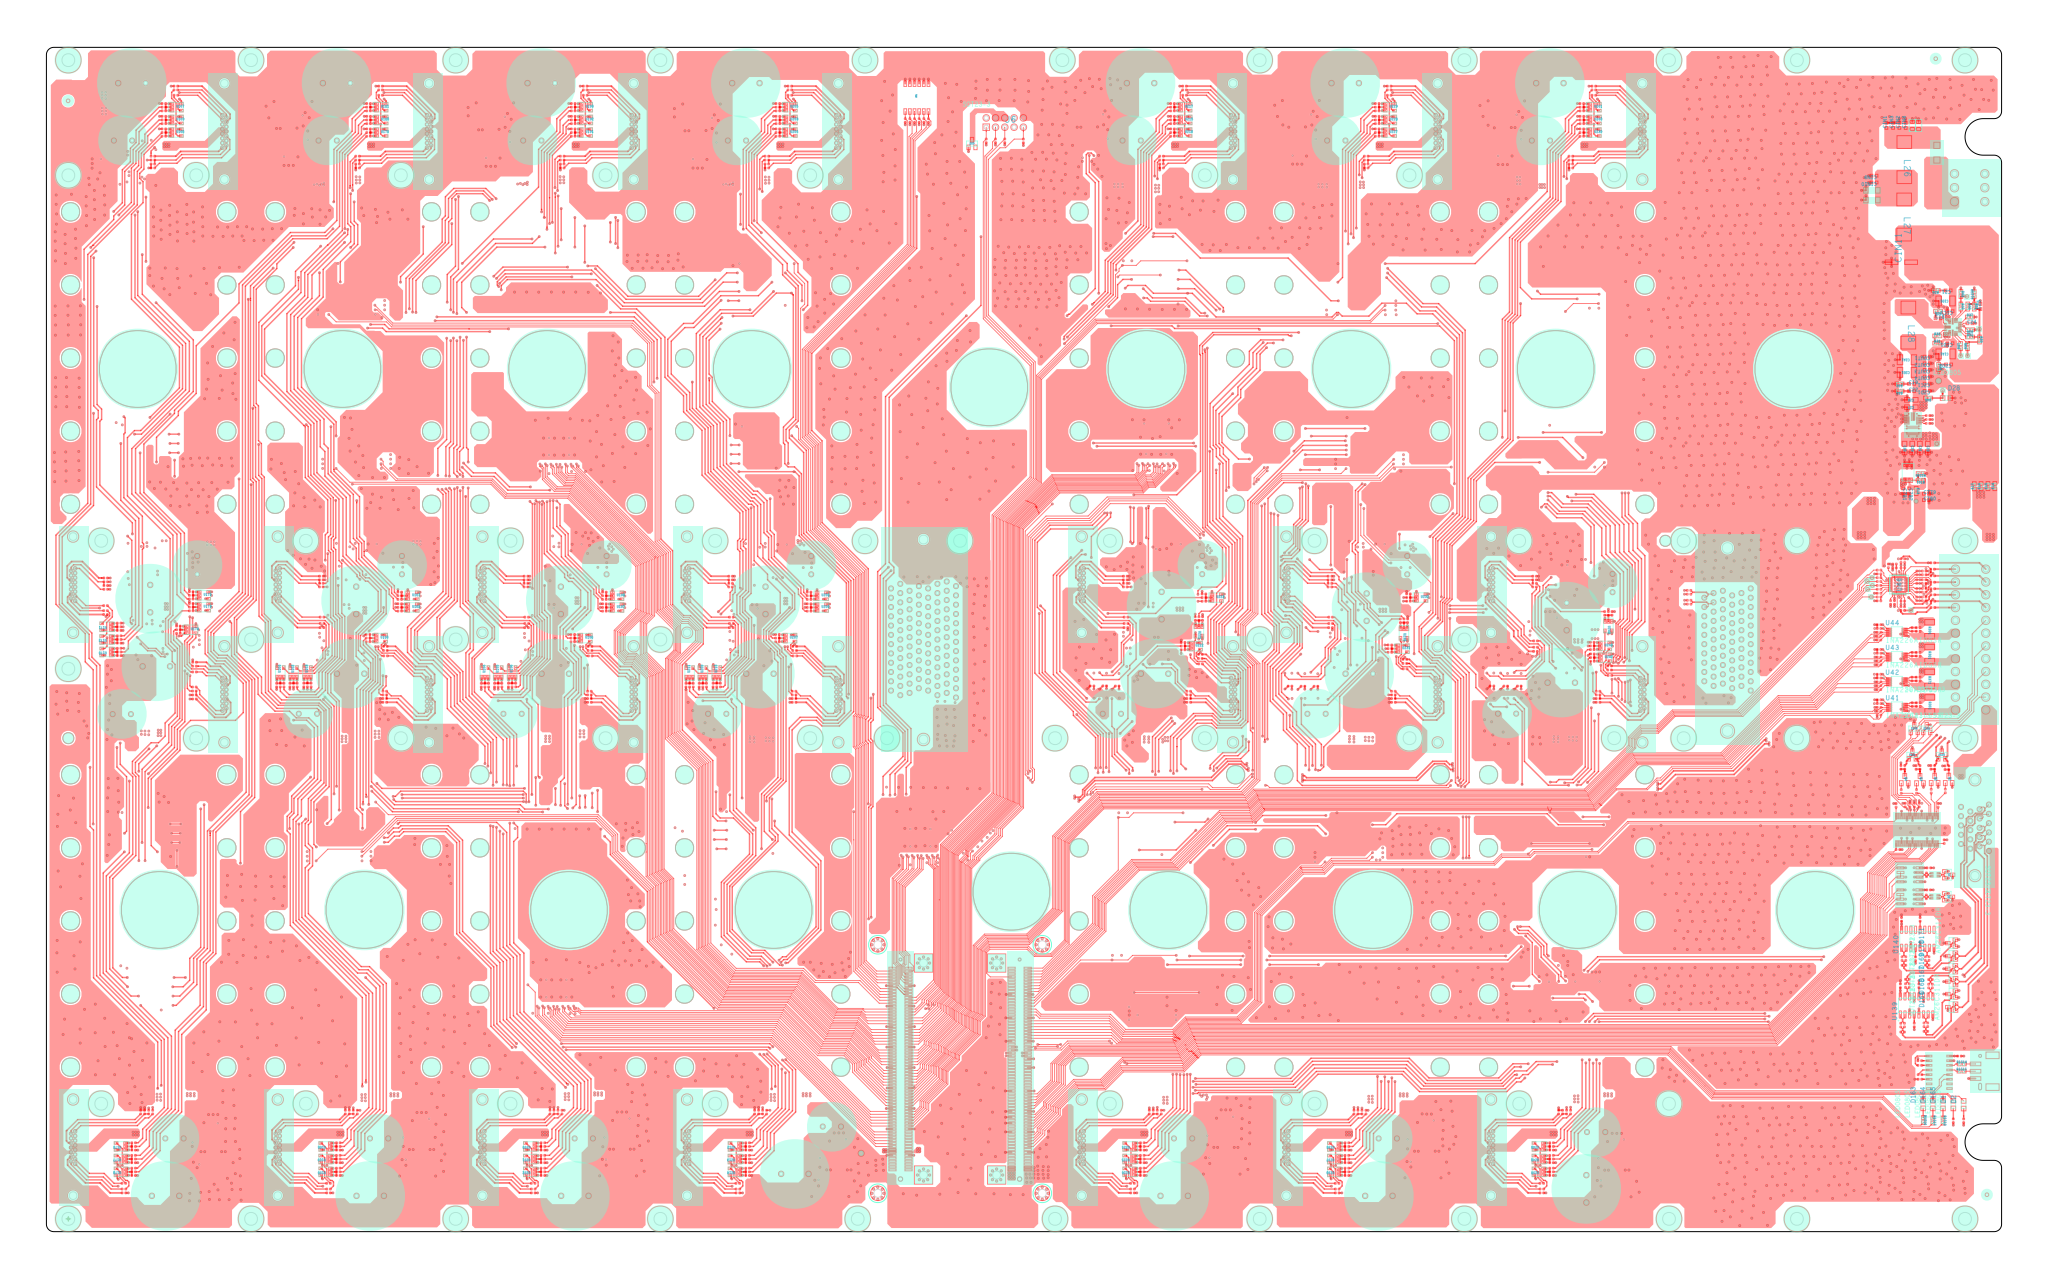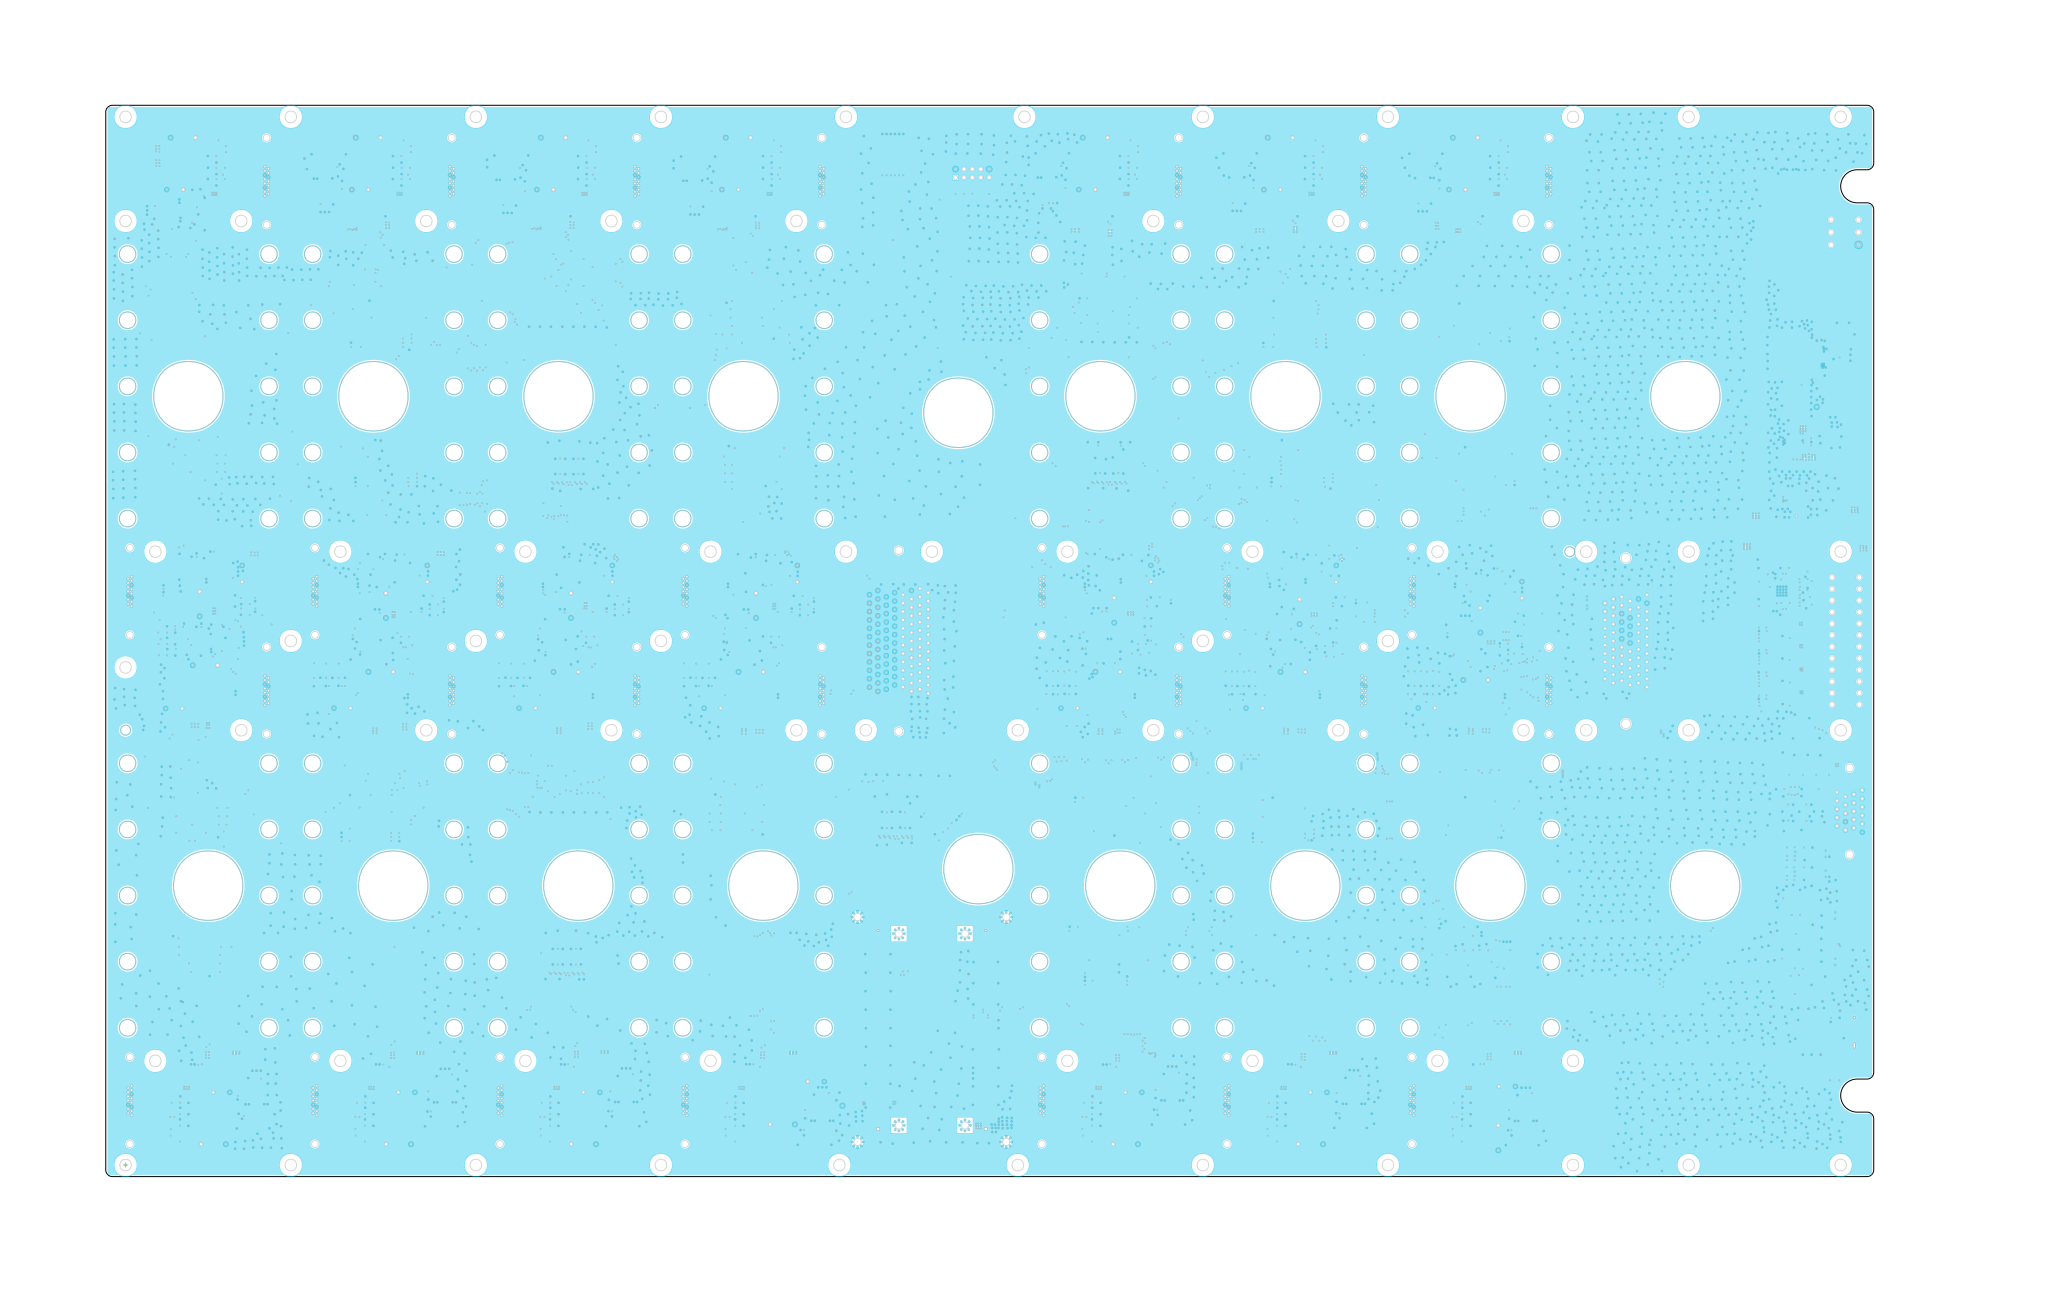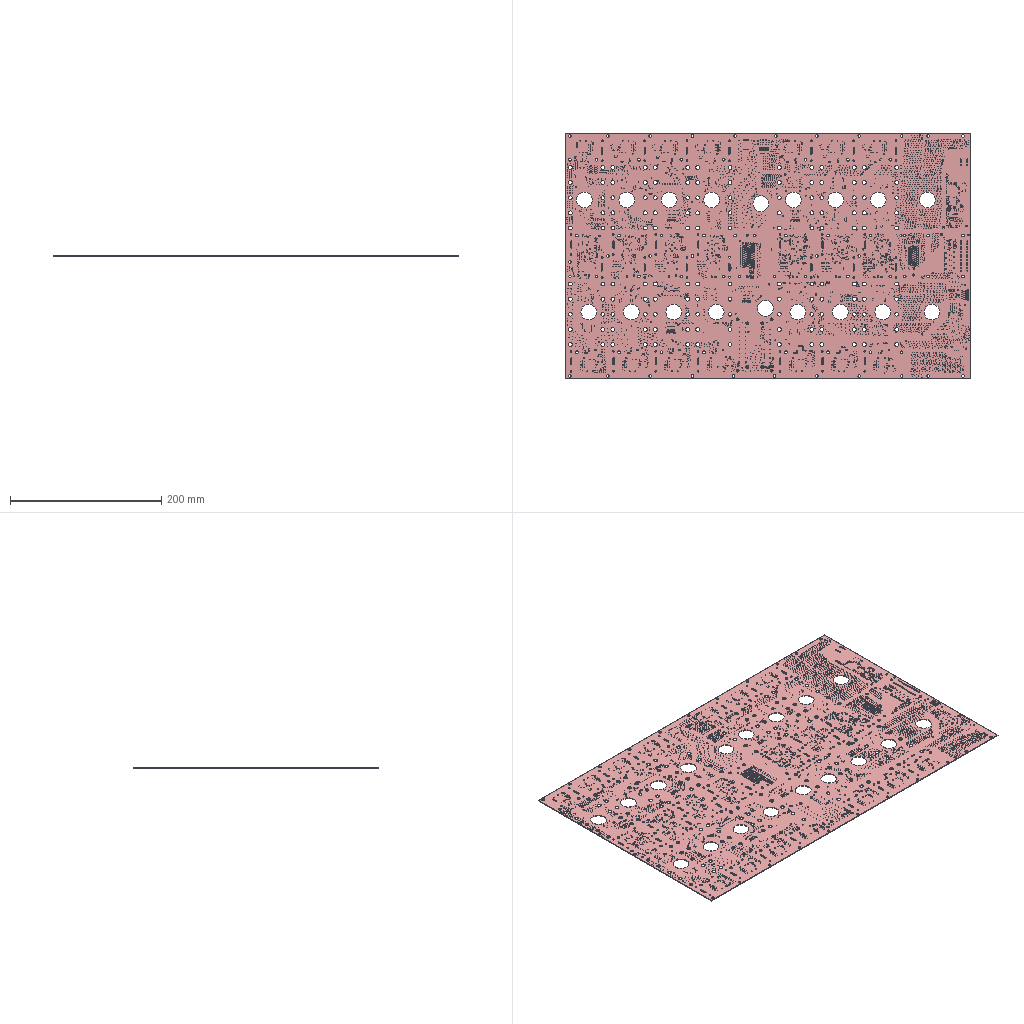Circuit board layout | Cadence Allegro | box 535 x 324 x 1.1 mm
Layer stack:
# Cadence Allegro layer stack of  (unit mm; from the constraint file cross-section; dielectric type: 0 not recorded (Allegro does not mark core vs prepreg), 3 surface material)
index,name,kind,layer,copper_thickness_mm,dielectric_type,dielectric_thickness_mm,dielectric_material,dielectric_constant
0,Top Surface,other,,,,,,
1,TOP,copper,TOP,0.0305,,,,
2,Dielectric1,dielectric,,,0,0.2032,FR-4,4.5
3,GND2,copper,GND2,0.0305,,,,
4,Dielectric2,dielectric,,,0,0.2032,FR-4,4.5
5,POWER3,copper,POWER3,0.0305,,,,
6,Dielectric3,dielectric,,,0,0.2032,FR-4,4.5
7,POWER4,copper,POWER4,0.0305,,,,
8,Dielectric4,dielectric,,,0,0.2032,FR-4,4.5
9,POWER5,copper,POWER5,0.0305,,,,
10,Dielectric5,dielectric,,,0,0.2032,FR-4,4.5
11,BOTTOM,copper,BOTTOM,0.0305,,,,
12,Bottom Surface,other,,,,,,
# drill layer pairs: low layer,high layer
drill_pair,TOP,BOTTOM
Part placement, first 387 of 2003 lines:
REFDES,COMP_VALUE,SYM_NAME,SYM_X,SYM_Y,SYM_ROTATE,SYM_MIRROR
C1A1,CAP/1210,1210,20223.830,9316.451,180.000,NO
C1B1,CAP/1210,1210,20223.389,9886.514,180.000,NO
C1C1,CAP/0603,0603C,20298.610,9776.349,180.000,NO
C1D1,CAP/0603,0603C,20298.007,9431.132,180.000,NO
C2A1,CAP/1210,1210,19807.074,9253.443,180.000,NO
C2B1,CAP/1210,1210,19807.330,9117.223,180.000,NO
C2C1,CAP/0603,0603C,20052.531,8995.668,180.000,NO
C2D1,CAP/0603,0603C,20052.775,8917.774,180.000,NO
C1,0.1uF/50V/10%/X7R/C0402,0402,20041.033,3543.170,0.000,NO
C2,0.1uF/50V/10%/X7R/C0402,0402,20043.132,3780.709,0.000,NO
C3,0.1uF/50V/10%/X7R/C0402,0402,9868.984,4088.897,270.000,YES
C18,CAP/0603,0603C,20115.669,9700.333,0.000,NO
C19,CAP/0603,0603C,19829.917,8993.392,0.000,NO
C20,CAP/0603,0603C,20283.645,9202.663,180.000,NO
C21,CAP/0603,0603C,20278.180,10000.317,180.000,NO
C22,CAP/0603,0603C,19830.114,8915.121,0.000,NO
C23,CAP/0603,0603C,20486.597,9521.519,270.000,YES
C24,CAP/0603,0603C,20458.586,9646.243,0.000,NO
C25,CAP/0603,0603C,20598.125,9799.148,90.000,NO
C26,22uF/10V/10%/X5R/C0805,0805,19854.448,8821.380,180.000,NO
C27,22uF/10V/10%/X5R/C0805,0805,19854.826,8741.998,180.000,NO
C28,22uF/10V/10%/X5R/C0805,0805,20031.984,8301.491,270.000,NO
C29,22uF/10V/10%/X5R/C0805,0805,19864.251,8301.979,270.000,NO
C30,22uF/10V/10%/X5R/C0805,0805,19781.180,8302.089,270.000,NO
C31,22uF/10V/10%/X5R/C0805,0805,19946.976,8301.695,270.000,NO
C32,39pF/6.3V/5%/NP0/C0402,0402,20033.570,8609.538,180.000,YES
C33,1uF/16V/10%/X5R/C0402,0402,11474.713,2195.292,180.000,YES
C34,0.1uF/50V/10%/X7R/C0402,0402,11474.670,2238.174,180.000,YES
C35,0.1uF/50V/10%/X7R/C0402,0402,11886.493,2245.548,180.000,YES
C58,0.1uF/50V/10%/X7R/C0402,0402,19783.543,5489.324,270.000,YES
C59,0.1uF/50V/10%/X7R/C0402,0402,19861.507,5539.147,270.000,NO
C60,0.1uF/50V/10%/X7R/C0402,0402,19782.094,5764.529,270.000,YES
C61,0.1uF/50V/10%/X7R/C0402,0402,19860.059,5814.351,270.000,NO
C62,0.1uF/50V/10%/X7R/C0402,0402,19782.488,6031.584,270.000,YES
C63,0.1uF/50V/10%/X7R/C0402,0402,19860.452,6081.407,270.000,NO
C64,0.1uF/50V/10%/X7R/C0402,0402,19782.228,6298.521,270.000,YES
C65,0.1uF/50V/10%/X7R/C0402,0402,19860.192,6348.344,270.000,NO
C66,0.1uF/50V/10%/X7R/C0402,0402,20005.038,4338.207,180.000,YES
C67,0.1uF/50V/10%/X7R/C0402,0402,19788.755,4338.274,180.000,YES
C68,0.1uF/50V/10%/X7R/C0402,0402,20044.216,4124.103,0.000,YES
C69,0.1uF/50V/10%/X7R/C0402,0402,19828.078,4132.560,0.000,YES
C70,10nF/50V/10%/X7R/C0402,0402,19741.669,6573.288,90.000,YES
C71,0.1uF/50V/10%/X7R/C0402,0402,19762.354,6653.458,0.000,NO
C72,10nF/50V/10%/X7R/C0402,0402,19781.252,6572.505,90.000,YES
C73,0.1uF/50V/10%/X7R/C0402,0402,19639.126,6881.029,180.000,YES
C74,1uF/50V/10%/X7R/C0402,0402,19639.066,6840.966,180.000,YES
C75,0.1uF/50V/10%/X7R/C0402,0402,19673.098,7011.800,180.000,NO
C76,1uF/50V/10%/X7R/C0402,0402,19672.937,7052.792,180.000,NO
C77,10nF/50V/10%/X7R/C0402,0402,19991.905,6657.611,180.000,YES
C78,0.1uF/50V/10%/X7R/C0402,0402,19913.314,6677.509,90.000,NO
C79,10nF/50V/10%/X7R/C0402,0402,19992.692,6697.194,180.000,YES
C80,0.1uF/50V/10%/X7R/C0402,0402,19607.204,7033.166,90.000,NO
C81,0.1uF/50V/10%/X7R/C0402,0402,19631.063,6638.962,270.000,NO
C82,0.1uF/50V/10%/X7R/C0402,0402,19673.039,6639.442,270.000,NO
C83,1uF/50V/10%/X7R/C0402,0402,19692.633,6737.348,180.000,YES
C84,10nF/50V/10%/X7R/C0402,0402,19991.905,6750.131,180.000,YES
C85,0.1uF/50V/10%/X7R/C0402,0402,19912.921,6770.029,90.000,NO
C86,10nF/50V/10%/X7R/C0402,0402,19992.692,6789.714,180.000,YES
C87,10nF/50V/10%/X7R/C0402,0402,19992.299,6937.533,180.000,YES
C88,0.1uF/50V/10%/X7R/C0402,0402,19913.708,6957.430,90.000,NO
C89,10nF/50V/10%/X7R/C0402,0402,19992.692,6977.513,180.000,YES
C92,10nF/50V/10%/X7R/C0402,0402,19782.755,7088.831,270.000,YES
C93,0.1uF/50V/10%/X7R/C0402,0402,19762.889,7011.930,180.000,NO
C94,10nF/50V/10%/X7R/C0402,0402,19743.208,7089.168,270.000,YES
C95,0.1uF/50V/10%/X7R/C0402,0402,19912.921,6864.127,90.000,NO
C96,10nF/50V/10%/X7R/C0402,0402,19991.118,6844.225,180.000,YES
C97,10nF/50V/10%/X7R/C0402,0402,19991.118,6883.832,0.000,NO
C601,0.1uF/50V/10%/X7R/C0402,0402,20371.975,1753.086,0.000,NO
C602,0.1uF/50V/10%/X7R/C0402,0402,19945.276,1653.380,0.000,NO
C603,0.1uF/50V/10%/X7R/C0402,0402,19945.018,1703.456,180.000,NO
C604,0.1uF/50V/10%/X7R/C0402,0402,19947.120,1503.787,0.000,NO
C605,0.1uF/50V/10%/X7R/C0402,0402,19947.589,1553.173,0.000,NO
C779,10uF/10V/10%/X5R/C0603,0603C,19989.640,7810.220,0.000,NO
C780,0.1uF/50V/10%/X7R/C0603,0603C,19989.640,7741.712,0.000,NO
C791,1uF/25V/10%/X7R/C0603,0603C,19767.594,7866.605,270.000,NO
C792,1uF/25V/10%/X7R/C0603,0603C,19832.562,7866.809,270.000,NO
C793,0.1uF/50V/10%/X7R/C0402,0402,19736.523,2510.286,90.000,NO
C794,0.1uF/50V/10%/X7R/C0402,0402,19748.804,3226.155,90.000,NO
C795,0.1uF/50V/10%/X7R/C0402,0402,16496.414,2609.012,270.000,YES
C796,0.1uF/50V/10%/X7R/C0402,0402,16233.607,2610.319,270.000,YES
C797,0.1uF/50V/10%/X7R/C0402,0402,15950.103,2608.174,270.000,YES
C798,0.1uF/50V/10%/X7R/C0402,0402,16105.874,2729.662,180.000,YES
C799,0.1uF/50V/10%/X7R/C0402,0402,558.788,4353.280,0.000,YES
C800,0.1uF/50V/10%/X7R/C0402,0402,584.410,2699.823,0.000,YES
C801,0.1uF/50V/10%/X7R/C0402,0402,534.906,8551.941,0.000,YES
C802,0.1uF/50V/10%/X7R/C0402,0402,7046.056,4386.111,0.000,YES
C803,0.1uF/50V/10%/X7R/C0402,0402,7179.477,10289.481,0.000,YES
C804,0.1uF/50V/10%/X7R/C0402,0402,7206.414,8535.630,0.000,YES
C805,0.1uF/50V/10%/X7R/C0402,0402,11407.186,10319.126,0.000,YES
C806,0.1uF/50V/10%/X7R/C0402,0402,11366.024,4373.528,0.000,YES
C807,0.1uF/50V/10%/X7R/C0402,0402,11295.063,2838.327,0.000,YES
C808,0.1uF/50V/10%/X7R/C0402,0402,16437.414,9808.681,180.000,YES
C809,0.1uF/50V/10%/X7R/C0402,0402,16370.079,3929.650,180.000,YES
C810,0.1uF/50V/10%/X7R/C0402,0402,16497.422,8097.280,180.000,YES
C811,0.1uF/50V/10%/X7R/C0402,0402,3423.780,8082.780,0.000,YES
C812,0.1uF/50V/10%/X7R/C0402,0402,14110.162,3844.087,0.000,YES
C813,0.1uF/50V/10%/X7R/C0402,0402,3211.040,3856.394,0.000,YES
C814,0.1uF/50V/10%/X7R/C0402,0402,14335.974,8080.960,0.000,YES
C815,0.1uF/50V/10%/X7R/C0402,0402,3359.607,9740.831,0.000,YES
C816,0.1uF/50V/10%/X7R/C0402,0402,14254.122,9737.953,0.000,YES
C817,0.1uF/50V/10%/X7R/C0402,0402,5394.308,8577.229,90.000,YES
C818,0.1uF/50V/10%/X7R/C0402,0402,5179.004,8581.733,90.000,YES
C819,0.1uF/50V/10%/X7R/C0402,0402,5394.969,8069.504,270.000,YES
C820,0.1uF/50V/10%/X7R/C0402,0402,5178.331,8073.492,270.000,YES
C821,0.1uF/50V/10%/X7R/C0402,0402,11828.107,8586.008,90.000,YES
C822,0.1uF/50V/10%/X7R/C0402,0402,11611.311,8587.028,90.000,YES
C823,0.1uF/50V/10%/X7R/C0402,0402,11827.276,8074.799,270.000,YES
C824,0.1uF/50V/10%/X7R/C0402,0402,11610.638,8078.788,270.000,YES
C825,0.1uF/50V/10%/X7R/C0402,0402,5365.749,2741.473,90.000,YES
C826,0.1uF/50V/10%/X7R/C0402,0402,5148.953,2742.492,90.000,YES
C827,0.1uF/50V/10%/X7R/C0402,0402,5364.918,2230.264,270.000,YES
C828,0.1uF/50V/10%/X7R/C0402,0402,5148.280,2234.252,270.000,YES
C829,0.1uF/50V/10%/X7R/C0402,0402,9286.972,4365.877,90.000,YES
C830,0.1uF/50V/10%/X7R/C0402,0402,9070.921,4367.893,90.000,YES
C831,0.1uF/50V/10%/X7R/C0402,0402,9070.248,3859.652,270.000,YES
C832,0.1uF/50V/10%/X7R/C0402,0402,9286.886,3855.664,270.000,YES
C833,0.1uF/50V/10%/X7R/C0402,0402,1029.527,11873.502,0.000,YES
C834,0.1uF/50V/10%/X7R/C0402,0402,1028.959,11738.009,0.000,YES
C835,0.1uF/50V/10%/X7R/C0402,0402,1028.945,12011.644,0.000,YES
C836,0.1uF/50V/10%/X7R/C0402,0402,547.436,6202.997,180.000,YES
C837,0.1uF/50V/10%/X7R/C0402,0402,546.904,6339.429,180.000,YES
C838,0.1uF/50V/10%/X7R/C0402,0402,547.436,6068.153,180.000,YES
C839,0.1uF/50V/10%/X7R/C0402,0402,1512.328,6606.945,90.000,YES
C840,0.1uF/50V/10%/X7R/C0402,0402,1374.048,6363.565,90.000,YES
C841,0.1uF/50V/10%/X7R/C0402,0402,1512.196,6733.853,90.000,YES
C842,0.1uF/50V/10%/X7R/C0402,0402,702.697,606.800,180.000,YES
C843,0.1uF/50V/10%/X7R/C0402,0402,703.347,468.846,180.000,YES
C844,0.1uF/50V/10%/X7R/C0402,0402,703.740,742.493,180.000,YES
C845,0.1uF/50V/10%/X7R/C0402,0402,3234.627,11873.502,0.000,YES
C846,0.1uF/50V/10%/X7R/C0402,0402,3234.045,12011.644,0.000,YES
C847,0.1uF/50V/10%/X7R/C0402,0402,3234.059,11738.009,0.000,YES
C848,0.1uF/50V/10%/X7R/C0402,0402,3758.492,6602.981,90.000,YES
C849,0.1uF/50V/10%/X7R/C0402,0402,3315.152,6272.937,90.000,YES
C850,0.1uF/50V/10%/X7R/C0402,0402,3760.076,6728.837,90.000,YES
C851,0.1uF/50V/10%/X7R/C0402,0402,2265.698,5834.736,180.000,YES
C852,0.1uF/50V/10%/X7R/C0402,0402,2408.361,5834.885,180.000,YES
C853,0.1uF/50V/10%/X7R/C0402,0402,2557.991,5835.767,180.000,YES
C854,0.1uF/50V/10%/X7R/C0402,0402,2908.572,742.457,180.000,YES
C855,0.1uF/50V/10%/X7R/C0402,0402,2907.529,606.764,180.000,YES
C856,0.1uF/50V/10%/X7R/C0402,0402,2908.179,468.810,180.000,YES
C857,0.1uF/50V/10%/X7R/C0402,0402,5439.207,11873.514,0.000,YES
C858,0.1uF/50V/10%/X7R/C0402,0402,5438.625,12011.656,0.000,YES
C859,0.1uF/50V/10%/X7R/C0402,0402,5438.639,11738.021,0.000,YES
C860,0.1uF/50V/10%/X7R/C0402,0402,4762.715,5835.275,180.000,YES
C861,0.1uF/50V/10%/X7R/C0402,0402,5519.876,6272.445,90.000,YES
C862,0.1uF/50V/10%/X7R/C0402,0402,4470.422,5834.244,180.000,YES
C863,0.1uF/50V/10%/X7R/C0402,0402,5963.216,6602.489,90.000,YES
C864,0.1uF/50V/10%/X7R/C0402,0402,4613.085,5834.393,180.000,YES
C865,0.1uF/50V/10%/X7R/C0402,0402,5964.800,6728.345,90.000,YES
C866,0.1uF/50V/10%/X7R/C0402,0402,5112.097,606.772,180.000,YES
C867,0.1uF/50V/10%/X7R/C0402,0402,5113.140,742.465,180.000,YES
C868,0.1uF/50V/10%/X7R/C0402,0402,5112.747,468.818,180.000,YES
C869,0.1uF/50V/10%/X7R/C0402,0402,7643.211,11738.021,0.000,YES
C870,0.1uF/50V/10%/X7R/C0402,0402,7643.779,11873.514,0.000,YES
C871,0.1uF/50V/10%/X7R/C0402,0402,7643.197,12011.656,0.000,YES
C872,0.1uF/50V/10%/X7R/C0402,0402,6967.435,5835.287,180.000,YES
C873,0.1uF/50V/10%/X7R/C0402,0402,6675.142,5834.256,180.000,YES
C874,0.1uF/50V/10%/X7R/C0402,0402,7724.596,6272.457,90.000,YES
C875,0.1uF/50V/10%/X7R/C0402,0402,8167.936,6602.501,90.000,YES
C876,0.1uF/50V/10%/X7R/C0402,0402,8169.520,6728.357,90.000,YES
C877,0.1uF/50V/10%/X7R/C0402,0402,6817.805,5834.405,180.000,YES
C878,0.1uF/50V/10%/X7R/C0402,0402,7316.937,606.516,180.000,YES
C879,0.1uF/50V/10%/X7R/C0402,0402,7317.587,468.562,180.000,YES
C880,0.1uF/50V/10%/X7R/C0402,0402,7317.980,742.209,180.000,YES
C881,0.1uF/50V/10%/X7R/C0402,0402,11895.299,11738.033,0.000,YES
C882,0.1uF/50V/10%/X7R/C0402,0402,11895.867,11873.526,0.000,YES
C883,0.1uF/50V/10%/X7R/C0402,0402,11895.285,12011.668,0.000,YES
C884,0.1uF/50V/10%/X7R/C0402,0402,12094.660,6186.713,90.000,YES
C885,0.1uF/50V/10%/X7R/C0402,0402,12196.924,6277.117,0.000,YES
C886,0.1uF/50V/10%/X7R/C0402,0402,11299.425,5738.603,180.000,NO
C887,0.1uF/50V/10%/X7R/C0402,0402,12423.692,6709.069,90.000,YES
C888,0.1uF/50V/10%/X7R/C0402,0402,11028.474,5739.592,180.000,NO
C889,0.1uF/50V/10%/X7R/C0402,0402,11164.603,5740.557,180.000,NO
C890,0.1uF/50V/10%/X7R/C0402,0402,11569.804,742.485,180.000,YES
C891,0.1uF/50V/10%/X7R/C0402,0402,11568.761,606.792,180.000,YES
C892,0.1uF/50V/10%/X7R/C0402,0402,11569.411,468.838,180.000,YES
C893,0.1uF/50V/10%/X7R/C0402,0402,14100.443,11873.534,0.000,YES
C894,0.1uF/50V/10%/X7R/C0402,0402,14099.875,11738.041,0.000,YES
C895,0.1uF/50V/10%/X7R/C0402,0402,14099.861,12011.676,0.000,YES
C896,0.1uF/50V/10%/X7R/C0402,0402,13161.162,5738.004,180.000,NO
C897,0.1uF/50V/10%/X7R/C0402,0402,14626.800,6709.717,90.000,YES
C898,0.1uF/50V/10%/X7R/C0402,0402,13300.527,5736.537,180.000,NO
C899,0.1uF/50V/10%/X7R/C0402,0402,13440.225,5736.203,180.000,NO
C900,0.1uF/50V/10%/X7R/C0402,0402,14322.484,6158.993,90.000,YES
C901,0.1uF/50V/10%/X7R/C0402,0402,14406.000,6253.705,0.000,YES
C902,0.1uF/50V/10%/X7R/C0402,0402,13774.504,742.229,180.000,YES
C903,0.1uF/50V/10%/X7R/C0402,0402,13773.461,606.536,180.000,YES
C904,0.1uF/50V/10%/X7R/C0402,0402,13774.111,468.582,180.000,YES
C905,0.1uF/50V/10%/X7R/C0402,0402,16305.271,11873.270,0.000,YES
C906,0.1uF/50V/10%/X7R/C0402,0402,16304.689,12011.412,0.000,YES
C907,0.1uF/50V/10%/X7R/C0402,0402,16304.703,11737.777,0.000,YES
C908,0.1uF/50V/10%/X7R/C0402,0402,15485.059,5738.173,180.000,NO
C909,0.1uF/50V/10%/X7R/C0402,0402,16608.108,6331.565,0.000,YES
C910,0.1uF/50V/10%/X7R/C0402,0402,15336.774,5739.640,180.000,NO
C911,0.1uF/50V/10%/X7R/C0402,0402,15631.237,5738.651,180.000,NO
C912,0.1uF/50V/10%/X7R/C0402,0402,16504.268,6062.561,90.000,YES
C913,0.1uF/50V/10%/X7R/C0402,0402,16605.204,6188.377,90.000,YES
C914,0.1uF/50V/10%/X7R/C0402,0402,15978.033,606.812,180.000,YES
C915,0.1uF/50V/10%/X7R/C0402,0402,15979.076,742.505,180.000,YES
C916,0.1uF/50V/10%/X7R/C0402,0402,15978.683,468.858,180.000,YES
C917,0.1uF/50V/10%/X7R/C0402,0402,792.932,11175.945,90.000,YES
C918,2pF/50V/10%/X7R/C0402,0402,699.080,11236.993,0.000,YES
C919,2pF/50V/10%/X7R/C0402,0402,699.864,11497.509,0.000,YES
C920,0.1uF/50V/10%/X7R/C0402,0402,304.672,11416.841,0.000,YES
C921,0.1uF/50V/10%/X7R/C0402,0402,820.324,7262.541,270.000,YES
C922,0.1uF/50V/10%/X7R/C0402,0402,1298.048,7017.737,180.000,YES
C923,2pF/50V/10%/X7R/C0402,0402,914.176,7196.773,180.000,YES
C924,2pF/50V/10%/X7R/C0402,0402,913.392,6937.069,180.000,YES
C925,0.1uF/50V/10%/X7R/C0402,0402,878.988,6426.733,270.000,YES
C926,0.1uF/50V/10%/X7R/C0402,0402,1366.688,586.357,0.000,YES
C927,0.1uF/50V/10%/X7R/C0402,0402,1609.904,1073.401,270.000,YES
C928,2pF/50V/10%/X7R/C0402,0402,1429.100,679.529,270.000,YES
C929,2pF/50V/10%/X7R/C0402,0402,1690.976,679.425,270.000,YES
C930,0.1uF/50V/10%/X7R/C0402,0402,1366.204,6184.709,180.000,YES
C931,2pF/50V/10%/X7R/C0402,0402,972.672,6363.985,180.000,YES
C932,2pF/50V/10%/X7R/C0402,0402,971.888,6104.149,180.000,YES
C933,0.1uF/50V/10%/X7R/C0402,0402,2575.444,11885.253,180.000,YES
C934,0.1uF/50V/10%/X7R/C0402,0402,3547.896,7019.189,180.000,YES
C935,0.1uF/50V/10%/X7R/C0402,0402,3068.684,7255.697,270.000,YES
C936,2pF/50V/10%/X7R/C0402,0402,3162.536,7198.093,180.000,YES
C937,2pF/50V/10%/X7R/C0402,0402,3161.752,6938.389,180.000,YES
C938,0.1uF/50V/10%/X7R/C0402,0402,2752.284,6113.205,0.000,YES
C939,0.1uF/50V/10%/X7R/C0402,0402,3614.840,610.869,0.000,YES
C940,0.1uF/50V/10%/X7R/C0402,0402,3855.332,1097.913,270.000,YES
C941,2pF/50V/10%/X7R/C0402,0402,3674.528,704.721,270.000,YES
C942,2pF/50V/10%/X7R/C0402,0402,3936.404,703.937,270.000,YES
C943,0.1uF/50V/10%/X7R/C0402,0402,2996.244,6595.385,270.000,YES
C944,2pF/50V/10%/X7R/C0402,0402,2816.396,6207.057,270.000,YES
C945,2pF/50V/10%/X7R/C0402,0402,3076.912,6206.273,270.000,YES
C946,0.1uF/50V/10%/X7R/C0402,0402,2323.768,11397.777,90.000,YES
C947,2pF/50V/10%/X7R/C0402,0402,2503.460,11791.217,90.000,YES
C948,2pF/50V/10%/X7R/C0402,0402,2242.944,11792.001,90.000,YES
C949,0.1uF/50V/10%/X7R/C0402,0402,4750.732,11870.145,180.000,YES
C950,0.1uF/50V/10%/X7R/C0402,0402,5750.384,7017.469,180.000,YES
C951,0.1uF/50V/10%/X7R/C0402,0402,5263.340,7257.961,270.000,YES
C952,2pF/50V/10%/X7R/C0402,0402,5357.192,7195.889,180.000,YES
C953,2pF/50V/10%/X7R/C0402,0402,5356.408,6936.397,180.000,YES
C954,0.1uF/50V/10%/X7R/C0402,0402,4962.176,6110.765,0.000,YES
C955,0.1uF/50V/10%/X7R/C0402,0402,5772.196,612.489,0.000,YES
C956,0.1uF/50V/10%/X7R/C0402,0402,6013.200,1100.385,270.000,YES
C957,2pF/50V/10%/X7R/C0402,0402,5832.564,706.341,270.000,YES
C958,2pF/50V/10%/X7R/C0402,0402,6093.760,705.557,270.000,YES
C959,0.1uF/50V/10%/X7R/C0402,0402,5202.668,6597.809,270.000,YES
C960,2pF/50V/10%/X7R/C0402,0402,5024.584,6203.937,270.000,YES
C961,2pF/50V/10%/X7R/C0402,0402,5283.740,6203.833,270.000,YES
C962,0.1uF/50V/10%/X7R/C0402,0402,4501.228,11383.441,90.000,YES
C963,2pF/50V/10%/X7R/C0402,0402,4679.988,11776.633,90.000,YES
C964,2pF/50V/10%/X7R/C0402,0402,4420.156,11777.417,90.000,YES
C965,0.1uF/50V/10%/X7R/C0402,0402,6729.612,11366.449,90.000,YES
C966,0.1uF/50V/10%/X7R/C0402,0402,7479.868,7255.525,270.000,YES
C967,0.1uF/50V/10%/X7R/C0402,0402,7962.860,7015.033,180.000,YES
C968,2pF/50V/10%/X7R/C0402,0402,7571.168,7193.793,180.000,YES
C969,2pF/50V/10%/X7R/C0402,0402,7572.764,6933.449,180.000,YES
C970,0.1uF/50V/10%/X7R/C0402,0402,7392.028,6594.201,270.000,YES
C971,0.1uF/50V/10%/X7R/C0402,0402,8350.832,876.805,270.000,YES
C972,0.1uF/50V/10%/X7R/C0402,0402,8061.516,390.441,0.000,YES
C973,2pF/50V/10%/X7R/C0402,0402,8169.856,482.593,270.000,YES
C974,2pF/50V/10%/X7R/C0402,0402,8431.392,482.149,270.000,YES
C975,0.1uF/50V/10%/X7R/C0402,0402,7151.536,6107.157,0.000,YES
C976,2pF/50V/10%/X7R/C0402,0402,7213.604,6201.353,270.000,YES
C977,2pF/50V/10%/X7R/C0402,0402,7473.100,6200.225,270.000,YES
C978,0.1uF/50V/10%/X7R/C0402,0402,6981.676,11857.917,180.000,YES
C979,2pF/50V/10%/X7R/C0402,0402,6909.740,11764.065,90.000,YES
C980,2pF/50V/10%/X7R/C0402,0402,6643.100,11764.849,90.000,YES
C981,0.1uF/50V/10%/X7R/C0402,0402,11189.860,11896.821,180.000,YES
C982,0.1uF/50V/10%/X7R/C0402,0402,11739.332,7236.017,180.000,YES
C983,0.1uF/50V/10%/X7R/C0402,0402,12207.984,7015.977,180.000,YES
C984,2pF/50V/10%/X7R/C0402,0402,11813.088,7196.101,180.000,YES
C985,2pF/50V/10%/X7R/C0402,0402,11812.304,6935.585,180.000,YES
C986,0.1uF/50V/10%/X7R/C0402,0402,11662.736,6611.225,270.000,YES
C987,0.1uF/50V/10%/X7R/C0402,0402,12272.164,632.629,0.000,YES
C988,0.1uF/50V/10%/X7R/C0402,0402,12518.780,1118.993,270.000,YES
C989,2pF/50V/10%/X7R/C0402,0402,12340.696,726.821,270.000,YES
C990,2pF/50V/10%/X7R/C0402,0402,12599.852,725.017,270.000,YES
C991,0.1uF/50V/10%/X7R/C0402,0402,11419.528,6123.161,0.000,YES
C992,2pF/50V/10%/X7R/C0402,0402,11480.576,6217.013,270.000,YES
C993,2pF/50V/10%/X7R/C0402,0402,11741.092,6216.229,270.000,YES
C994,0.1uF/50V/10%/X7R/C0402,0402,10949.368,11409.777,90.000,YES
C995,2pF/50V/10%/X7R/C0402,0402,11127.796,11803.649,90.000,YES
C996,2pF/50V/10%/X7R/C0402,0402,10868.296,11803.753,90.000,YES
C997,0.1uF/50V/10%/X7R/C0402,0402,13433.856,11894.801,180.000,YES
C998,0.1uF/50V/10%/X7R/C0402,0402,14403.352,7015.037,180.000,YES
C999,0.1uF/50V/10%/X7R/C0402,0402,13924.412,7254.717,270.000,YES
C1000,2pF/50V/10%/X7R/C0402,0402,14014.212,7193.801,180.000,YES
C1001,2pF/50V/10%/X7R/C0402,0402,14013.832,6933.965,180.000,YES
C1002,0.1uF/50V/10%/X7R/C0402,0402,13894.836,6601.701,270.000,YES
C1003,0.1uF/50V/10%/X7R/C0402,0402,14683.836,1079.149,270.000,YES
C1004,0.1uF/50V/10%/X7R/C0402,0402,14440.964,591.425,0.000,YES
C1005,2pF/50V/10%/X7R/C0402,0402,14502.696,685.277,270.000,YES
C1006,2pF/50V/10%/X7R/C0402,0402,14764.908,684.493,270.000,YES
C1007,0.1uF/50V/10%/X7R/C0402,0402,13654.344,6114.657,0.000,YES
C1008,2pF/50V/10%/X7R/C0402,0402,13715.392,6208.509,270.000,YES
C1009,2pF/50V/10%/X7R/C0402,0402,13975.908,6207.725,270.000,YES
C1010,0.1uF/50V/10%/X7R/C0402,0402,13189.384,11408.165,90.000,YES
C1011,2pF/50V/10%/X7R/C0402,0402,13367.812,11801.357,90.000,YES
C1012,2pF/50V/10%/X7R/C0402,0402,13108.312,11802.141,90.000,YES
C1013,0.1uF/50V/10%/X7R/C0402,0402,15402.788,11404.073,90.000,YES
C1014,0.1uF/50V/10%/X7R/C0402,0402,16125.148,7061.833,270.000,YES
C1015,0.1uF/50V/10%/X7R/C0402,0402,16593.956,6822.149,180.000,YES
C1016,2pF/50V/10%/X7R/C0402,0402,16207.248,7000.573,180.000,YES
C1017,2pF/50V/10%/X7R/C0402,0402,16207.276,6741.481,180.000,YES
C1018,0.1uF/50V/10%/X7R/C0402,0402,16036.216,6520.621,270.000,YES
C1019,0.1uF/50V/10%/X7R/C0402,0402,16490.472,386.793,0.000,YES
C1020,0.1uF/50V/10%/X7R/C0402,0402,16731.304,874.517,270.000,YES
C1021,2pF/50V/10%/X7R/C0402,0402,16551.520,480.645,270.000,YES
C1022,2pF/50V/10%/X7R/C0402,0402,16812.036,479.861,270.000,YES
C1023,0.1uF/50V/10%/X7R/C0402,0402,15795.384,6029.833,0.000,YES
C1024,2pF/50V/10%/X7R/C0402,0402,15856.432,6123.685,270.000,YES
C1025,2pF/50V/10%/X7R/C0402,0402,16116.948,6122.901,270.000,YES
C1026,0.1uF/50V/10%/X7R/C0402,0402,15645.652,11891.965,180.000,YES
C1027,2pF/50V/10%/X7R/C0402,0402,15584.940,11799.469,90.000,YES
C1028,2pF/50V/10%/X7R/C0402,0402,15322.392,11798.897,90.000,YES
C1029,10nF/50V/10%/X7R/C0402,0402,19788.565,4456.362,270.000,YES
C1030,10nF/50V/10%/X7R/C0402,0402,19838.199,4456.111,270.000,YES
C1031,10nF/50V/10%/X7R/C0402,0402,19887.066,4456.249,270.000,YES
C1032,10nF/50V/10%/X7R/C0402,0402,19939.960,4456.572,270.000,YES
CIN1,CAP/0603,0603C,19585.853,11750.434,90.000,NO
CIN2,CAP/0603,0603C,19725.699,11750.663,90.000,NO
CIN3,CAP/0603,0603C,19657.731,11750.789,90.000,NO
CIN4,CAP/0603,0603C,19793.996,11749.784,90.000,NO
CIN5,CAP/0603,0805C,19865.661,11777.486,90.000,NO
CIN6,CAP/0603,0805C,19932.070,11776.305,90.000,NO
CIN7,CAP/0603,1206,19428.965,11077.666,180.000,NO
CIN8,CAP/0603,1206,19429.622,10973.675,180.000,NO
CIN9,CAP/0603,0603C,19479.440,11236.036,180.000,NO
CIN10,CAP/0603,0603C,19480.148,11162.654,180.000,NO
CIN11,CAP/ELECT/DIP/OD5.3P2.0,AP-SMD_BD6_3-L6_6-W6_6-LS7_21,19746.802,10303.861,180.000,NO
CIN12,ECF1HM182M27OTPO,AP-SMD_BD18-L27-W6_6-LS7_21,684.709,12232.603,270.000,NO
CIN13,ECF1JM331G20OTPO,AP-SMD_BD10-L20-W6_6-LS7_21,588.772,11614.355,270.000,NO
CIN14,ECF1HM182M27OTPO,AP-SMD_BD18-L27-W6_6-LS7_21,881.914,6680.307,0.000,NO
CIN15,ECF1JM331G20OTPO,AP-SMD_BD10-L20-W6_6-LS7_21,1388.626,7040.910,180.000,NO
CIN16,ECF1HM182M27OTPO,AP-SMD_BD18-L27-W6_6-LS7_21,947.788,5950.744,270.000,NO
CIN17,ECF1JM331G20OTPO,AP-SMD_BD10-L20-W6_6-LS7_21,575.662,5436.268,270.000,NO
CIN18,ECF1HM182M27OTPO,AP-SMD_BD18-L27-W6_6-LS7_21,1047.351,247.831,90.000,NO
CIN19,ECF1JM331G20OTPO,AP-SMD_BD10-L20-W6_6-LS7_21,1143.288,866.079,90.000,NO
CIN20,ECF1HM182M27OTPO,AP-SMD_BD18-L27-W6_6-LS7_21,2889.809,12232.603,270.000,NO
CIN21,ECF1JM331G20OTPO,AP-SMD_BD10-L20-W6_6-LS7_21,2793.872,11614.355,270.000,NO
CIN22,ECF1HM182M27OTPO,AP-SMD_BD18-L27-W6_6-LS7_21,3101.180,6661.813,0.000,NO
CIN23,ECF1JM331G20OTPO,AP-SMD_BD10-L20-W6_6-LS7_21,3593.540,7041.044,180.000,NO
CIN24,ECF1JM331G20OTPO,AP-SMD_BD10-L20-W6_6-LS7_21,2580.835,5440.351,270.000,NO
CIN25,ECF1HM182M27OTPO,AP-SMD_BD18-L27-W6_6-LS7_21,3041.012,5872.040,270.000,NO
CIN26,ECF1HM182M27OTPO,AP-SMD_BD18-L27-W6_6-LS7_21,3252.183,247.795,90.000,NO
CIN27,ECF1JM331G20OTPO,AP-SMD_BD10-L20-W6_6-LS7_21,3348.120,866.043,90.000,NO
CIN28,ECF1HM182M27OTPO,AP-SMD_BD18-L27-W6_6-LS7_21,5094.389,12232.615,270.000,NO
CIN29,ECF1JM331G20OTPO,AP-SMD_BD10-L20-W6_6-LS7_21,4998.452,11614.367,270.000,NO
CIN30,ECF1HM182M27OTPO,AP-SMD_BD18-L27-W6_6-LS7_21,5305.904,6661.321,0.000,NO
CIN31,ECF1JM331G20OTPO,AP-SMD_BD10-L20-W6_6-LS7_21,5798.264,7040.552,180.000,NO
CIN32,ECF1HM182M27OTPO,AP-SMD_BD18-L27-W6_6-LS7_21,5245.736,5871.548,270.000,NO
CIN33,ECF1JM331G20OTPO,AP-SMD_BD10-L20-W6_6-LS7_21,4785.559,5439.859,270.000,NO
CIN34,ECF1HM182M27OTPO,AP-SMD_BD18-L27-W6_6-LS7_21,5456.751,247.803,90.000,NO
CIN35,ECF1JM331G20OTPO,AP-SMD_BD10-L20-W6_6-LS7_21,5552.688,866.051,90.000,NO
CIN36,ECF1HM182M27OTPO,AP-SMD_BD18-L27-W6_6-LS7_21,7298.961,12232.615,270.000,NO
CIN37,ECF1JM331G20OTPO,AP-SMD_BD10-L20-W6_6-LS7_21,7203.024,11614.367,270.000,NO
CIN38,ECF1JM331G20OTPO,AP-SMD_BD10-L20-W6_6-LS7_21,6990.279,5439.871,270.000,NO
CIN39,ECF1HM182M27OTPO,AP-SMD_BD18-L27-W6_6-LS7_21,7450.456,5871.560,270.000,NO
CIN40,ECF1JM331G20OTPO,AP-SMD_BD10-L20-W6_6-LS7_21,8002.984,7040.564,180.000,NO
CIN41,ECF1HM182M27OTPO,AP-SMD_BD18-L27-W6_6-LS7_21,7510.624,6661.333,0.000,NO
CIN42,ECF1HM182M27OTPO,AP-SMD_BD18-L27-W6_6-LS7_21,7826.575,484.451,90.000,NO
CIN43,ECF1JM331G20OTPO,AP-SMD_BD10-L20-W6_6-LS7_21,8225.584,994.083,90.000,NO
CIN44,ECF1HM182M27OTPO,AP-SMD_BD18-L27-W6_6-LS7_21,11551.049,12232.627,270.000,NO
CIN45,ECF1JM331G20OTPO,AP-SMD_BD10-L20-W6_6-LS7_21,11455.112,11614.379,270.000,NO
CIN46,ECF1HM182M27OTPO,AP-SMD_BD18-L27-W6_6-LS7_21,11777.764,6605.569,0.000,NO
CIN47,ECF1JM331G20OTPO,AP-SMD_BD10-L20-W6_6-LS7_21,12215.016,7042.344,180.000,NO
CIN48,ECF1HM182M27OTPO,AP-SMD_BD18-L27-W6_6-LS7_21,11702.196,5871.720,270.000,NO
CIN49,ECF1JM331G20OTPO,AP-SMD_BD10-L20-W6_6-LS7_21,11242.019,5440.031,270.000,NO
CIN50,ECF1HM182M27OTPO,AP-SMD_BD18-L27-W6_6-LS7_21,11913.415,247.823,90.000,NO
CIN51,ECF1JM331G20OTPO,AP-SMD_BD10-L20-W6_6-LS7_21,12009.352,866.071,90.000,NO
CIN52,ECF1JM331G20OTPO,AP-SMD_BD10-L20-W6_6-LS7_21,13659.688,11614.387,270.000,NO
CIN53,ECF1HM182M27OTPO,AP-SMD_BD18-L27-W6_6-LS7_21,13755.625,12232.635,270.000,NO
CIN54,ECF1JM331G20OTPO,AP-SMD_BD10-L20-W6_6-LS7_21,13446.747,5439.871,270.000,NO
CIN55,ECF1HM182M27OTPO,AP-SMD_BD18-L27-W6_6-LS7_21,13906.924,5871.560,270.000,NO
CIN56,ECF1HM182M27OTPO,AP-SMD_BD18-L27-W6_6-LS7_21,13986.544,6588.393,0.000,NO
CIN57,ECF1JM331G20OTPO,AP-SMD_BD10-L20-W6_6-LS7_21,14423.792,7040.564,180.000,NO
CIN58,ECF1HM182M27OTPO,AP-SMD_BD18-L27-W6_6-LS7_21,14118.115,247.567,90.000,NO
CIN59,ECF1JM331G20OTPO,AP-SMD_BD10-L20-W6_6-LS7_21,14214.052,865.815,90.000,NO
CIN60,ECF1HM182M27OTPO,AP-SMD_BD18-L27-W6_6-LS7_21,15960.453,12232.371,270.000,NO
CIN61,ECF1JM331G20OTPO,AP-SMD_BD10-L20-W6_6-LS7_21,15864.516,11614.123,270.000,NO
CIN62,ECF1HM182M27OTPO,AP-SMD_BD18-L27-W6_6-LS7_21,16083.440,5775.124,270.000,NO
CIN63,ECF1JM331G20OTPO,AP-SMD_BD10-L20-W6_6-LS7_21,15499.271,5441.503,270.000,NO
CIN64,ECF1HM182M27OTPO,AP-SMD_BD18-L27-W6_6-LS7_21,16141.172,6487.097,0.000,NO
CIN65,ECF1JM331G20OTPO,AP-SMD_BD10-L20-W6_6-LS7_21,16635.484,6847.980,180.000,NO
CIN66,ECF1HM182M27OTPO,AP-SMD_BD18-L27-W6_6-LS7_21,16353.540,323.173,0.000,NO
CIN67,ECF1JM331G20OTPO,AP-SMD_BD10-L20-W6_6-LS7_21,16458.807,934.695,90.000,NO
COUT1,CAP/0603,0603C,20053.369,9286.518,180.000,NO
COUT2,CAP/0603,0603C,20052.976,9214.628,180.000,NO
COUT3,CAP/0603,0603C,20053.369,9143.967,180.000,NO
Pad and via stacks, first 109 of 126 lines:
# Allegro (Cadence) via spans and padstacks; design units: ("mils" 3 1000)
# via spans: padstack,start_layer,end_layer,net_example,count
VIA12X20,ETCH/TOP,ETCH/BOTTOM,AGND,6280
VIA12X20,ETCH/BOTTOM,ETCH/TOP,VCC5V,40
# Allegro padstack definitions: name,start_layer,end_layer,drill,plating,holeType,type
2020B,"ETCH/TOP","ETCH/TOP",0.0,"PLATED","none","smd"
SMD_R551X500P0S40,"ETCH/TOP","ETCH/TOP",0.0,"PLATED","none","smd"
PSM_065X081R,"ETCH/TOP","ETCH/TOP",0.0,"PLATED","none","smd"
SMD50_50,"ETCH/TOP","ETCH/TOP",0.0,"PLATED","none","smd"
SMD200X50,"ETCH/TOP","ETCH/TOP",0.0,"PLATED","none","smd"
R75X85,"ETCH/TOP","ETCH/TOP",0.0,"NON_PLATED","none","smd"
RE55X40,"ETCH/TOP","ETCH/TOP",0.0,"NON_PLATED","none","smd"
SMD_R591X1063P0S40,"ETCH/TOP","ETCH/TOP",0.0,"PLATED","none","smd"
Y10,"ETCH/TOP","ETCH/TOP",0.0,"NON_PLATED","none","smd"
R61X15,"ETCH/TOP","ETCH/TOP",0.0,"NON_PLATED","none","smd"
SMD_S50P0S40,"ETCH/TOP","ETCH/TOP",0.0,"PLATED","none","smd"
SMD_R510X80P0S0,"ETCH/TOP","ETCH/TOP",0.0,"PLATED","none","smd"
SMD_R810X100P0S0,"ETCH/TOP","ETCH/TOP",0.0,"PLATED","none","smd"
S_R147T28D2M147_28P147_28,"ETCH/TOP","ETCH/TOP",0.0,"PLATED","none","smd"
R150_30_K,"ETCH/TOP","ETCH/TOP",0.0,"NON_PLATED","none","smd"
RX148Y148D0T,"ETCH/TOP","ETCH/TOP",0.0,"PLATED","none","smd"
RX10Y32D0T,"ETCH/TOP","ETCH/TOP",0.0,"PLATED","none","smd"
SMD36_50,"ETCH/TOP","ETCH/TOP",0.0,"PLATED","none","smd"
PSM_091S_PM,"ETCH/TOP","ETCH/TOP",0.0,"NON_PLATED","none","smd"
R105_100,"ETCH/TOP","ETCH/TOP",0.0,"PLATED","none","smd"
BGA10_SMD0X619,"ETCH/TOP","ETCH/TOP",0.0,"NON_PLATED","none","smd"
O0R9X1R4,"ETCH/TOP","ETCH/TOP",0.0,"NON_PLATED","none","smd"
R127X152,"ETCH/TOP","ETCH/TOP",0.0,"NON_PLATED","none","smd"
SMD_R1378X472P0S20,"ETCH/TOP","ETCH/TOP",0.0,"PLATED","none","smd"
SMD_R600X300P0S20,"ETCH/TOP","ETCH/TOP",0.0,"PLATED","none","smd"
SMD_R1378X1575P0S20,"ETCH/TOP","ETCH/TOP",0.0,"PLATED","none","smd"
RX43Y10D0T,"ETCH/TOP","ETCH/TOP",0.0,"PLATED","none","smd"
RX59Y10D0T,"ETCH/TOP","ETCH/TOP",0.0,"PLATED","none","smd"
RX5Y5D0T,"ETCH/TOP","ETCH/TOP",0.0,"PLATED","none","smd"
RX28Y10D0T,"ETCH/TOP","ETCH/TOP",0.0,"PLATED","none","smd"
SMD_S300P0S10,"ETCH/TOP","ETCH/TOP",0.0,"PLATED","none","smd"
Y3_MARK,"ETCH/TOP","ETCH/TOP",0.0,"PLATED","none","smd"
F45,"ETCH/TOP","ETCH/TOP",0.0,"PLATED","none","smd"
R91X127,"ETCH/TOP","ETCH/TOP",0.0,"NON_PLATED","none","smd"
S91,"ETCH/TOP","ETCH/TOP",0.0,"NON_PLATED","none","smd"
R127X120,"ETCH/TOP","ETCH/TOP",0.0,"NON_PLATED","none","smd"
R40X36,"ETCH/TOP","ETCH/TOP",0.0,"PLATED","none","smd"
R127X121,"ETCH/TOP","ETCH/TOP",0.0,"PLATED","none","smd"
R88X76,"ETCH/TOP","ETCH/TOP",0.0,"PLATED","none","smd"
R60X20,"ETCH/TOP","ETCH/TOP",0.0,"PLATED","none","smd"
R120X70,"ETCH/TOP","ETCH/TOP",0.0,"PLATED","none","smd"
R50X32,"ETCH/TOP","ETCH/TOP",0.0,"PLATED","none","smd"
S437,"ETCH/TOP","ETCH/TOP",0.0,"PLATED","none","smd"
Y4,"ETCH/TOP","ETCH/TOP",0.0,"PLATED","none","smd"
SMD0_45R,"ETCH/TOP","ETCH/TOP",0.0,"PLATED","none","smd"
R85X65,"ETCH/TOP","ETCH/TOP",0.0,"PLATED","none","smd"
Y50,"ETCH/TOP","ETCH/TOP",0.0,"PLATED","none","smd"
RE43_31X19_68,"ETCH/TOP","ETCH/TOP",0.0,"PLATED","none","smd"
RE134X170,"ETCH/TOP","ETCH/TOP",0.0,"PLATED","none","smd"
SMD_R98X276P0S30,"ETCH/TOP","ETCH/TOP",0.0,"PLATED","none","smd"
SMD_R98X433P0S30,"ETCH/TOP","ETCH/TOP",0.0,"PLATED","none","smd"
SMD_R98X276P0S10,"ETCH/TOP","ETCH/TOP",0.0,"PLATED","none","smd"
SMD_R98X433P0S10,"ETCH/TOP","ETCH/TOP",0.0,"PLATED","none","smd"
SMD_R236X669P0S40,"ETCH/TOP","ETCH/TOP",0.0,"PLATED","none","smd"
SMD_R236X669P0S30,"ETCH/TOP","ETCH/TOP",0.0,"PLATED","none","smd"
SMD_R98X433S30,"ETCH/TOP","ETCH/TOP",0.0,"PLATED","none","smd"
C12_6,"ETCH/TOP","ETCH/TOP",0.0,"PLATED","none","smd"
R80X25,"ETCH/TOP","ETCH/TOP",0.0,"PLATED","none","smd"
SMD10_61,"ETCH/TOP","ETCH/TOP",0.0,"PLATED","none","smd"
R29_92X50,"ETCH/TOP","ETCH/TOP",0.0,"PLATED","none","smd"
S_R197T60D5M197_60P197_60,"ETCH/TOP","ETCH/TOP",0.0,"PLATED","none","smd"
R36X18,"ETCH/TOP","ETCH/TOP",0.0,"PLATED","none","smd"
R29X10,"ETCH/TOP","ETCH/TOP",0.0,"PLATED","none","smd"
R45X150,"ETCH/TOP","ETCH/TOP",0.0,"NON_PLATED","none","smd"
S17,"ETCH/TOP","ETCH/TOP",0.0,"NON_PLATED","none","smd"
R165X317,"ETCH/TOP","ETCH/TOP",0.0,"NON_PLATED","none","smd"
RE39_37X27_56,"ETCH/TOP","ETCH/TOP",0.0,"NON_PLATED","none","smd"
S_R157T41D2M157_41P157_41,"ETCH/TOP","ETCH/TOP",0.0,"PLATED","none","smd"
PAD18,"ETCH/TOP","ETCH/TOP",0.0,"NON_PLATED","none","smd"
Y24,"ETCH/TOP","ETCH/BOTTOM",51.181,"PLATED","circle_drill","through"
C68_11D35,"ETCH/TOP","ETCH/BOTTOM",35.039,"PLATED","circle_drill","through"
SQ68_11D35,"ETCH/TOP","ETCH/BOTTOM",35.039,"PLATED","circle_drill","through"
C130D130N,"ETCH/TOP","ETCH/BOTTOM",129.921,"NON_PLATED","circle_drill","through"
C98D70_87,"ETCH/TOP","ETCH/BOTTOM",70.87,"PLATED","circle_drill","through"
C70_87D51_18,"ETCH/TOP","ETCH/BOTTOM",51.181,"PLATED","circle_drill","through"
C60D40,"ETCH/TOP","ETCH/BOTTOM",40.0,"PLATED","circle_drill","through"
Y0_80,"ETCH/TOP","ETCH/BOTTOM",31.496,"NON_PLATED","circle_drill","through"
Y0_120,"ETCH/TOP","ETCH/BOTTOM",47.244,"NON_PLATED","circle_drill","through"
Y60,"ETCH/TOP","ETCH/BOTTOM",123.622,"PLATED","circle_drill","through"
Y0_0_6,"ETCH/TOP","ETCH/BOTTOM",23.622,"PLATED","circle_drill","through"
Y1000,"ETCH/TOP","ETCH/BOTTOM",39.37,"PLATED","circle_drill","through"
Y3000,"ETCH/TOP","ETCH/BOTTOM",78.74,"PLATED","circle_drill","through"
VIA24D12,"ETCH/TOP","ETCH/BOTTOM",12.0,"PLATED","circle_drill","through"
Y4_6,"ETCH/TOP","ETCH/BOTTOM",86.614,"PLATED","circle_drill","through"
F152,"ETCH/TOP","ETCH/BOTTOM",40.0,"PLATED","circle_drill","through"
F15,"ETCH/TOP","ETCH/BOTTOM",40.0,"PLATED","circle_drill","through"
Y150_1,"ETCH/TOP","ETCH/BOTTOM",59.055,"PLATED","circle_drill","through"
Y70_120_1,"ETCH/TOP","ETCH/BOTTOM",27.559,"PLATED","circle_drill","through"
D3,"ETCH/TOP","ETCH/BOTTOM",118.11,"NON_PLATED","circle_drill","through"
Y328,"ETCH/TOP","ETCH/BOTTOM",129.134,"NON_PLATED","circle_drill","through"
Y300_1,"ETCH/TOP","ETCH/BOTTOM",125.0,"NON_PLATED","circle_drill","through"
Y4_5,"ETCH/TOP","ETCH/BOTTOM",86.614,"PLATED","circle_drill","through"
VIA_D10C020,"ETCH/TOP","ETCH/BOTTOM",10.0,"PLATED","circle_drill","through"
EX63Y63D43P,"ETCH/TOP","ETCH/BOTTOM",43.0,"PLATED","circle_drill","through"
EX83Y83D63P,"ETCH/TOP","ETCH/BOTTOM",63.0,"PLATED","circle_drill","through"
T18X9,"ETCH/TOP","ETCH/BOTTOM",31.496,"NON_PLATED","oval slot","through"
Y8,"ETCH/TOP","ETCH/BOTTOM",31.496,"NON_PLATED","circle_drill","through"
VIA12_24,"ETCH/TOP","ETCH/BOTTOM",11.811,"PLATED","circle_drill","through"
VIA12X20,"ETCH/TOP","ETCH/BOTTOM",12.0,"PLATED","circle_drill","through"
HOLE2-3_5,"ETCH/TOP","ETCH/BOTTOM",82.681,"PLATED","circle_drill","through"
HOLELOCK_2P3_MM,"ETCH/TOP","ETCH/BOTTOM",98.425,"PLATED","circle_drill","through"
PAD36CIR26D_1,"ETCH/TOP","ETCH/BOTTOM",26.0,"PLATED","circle_drill","through"
PAD36SQ26D_1,"ETCH/TOP","ETCH/BOTTOM",26.0,"PLATED","circle_drill","through"
Y100_1,"ETCH/TOP","ETCH/BOTTOM",39.37,"NON_PLATED","circle_drill","through"